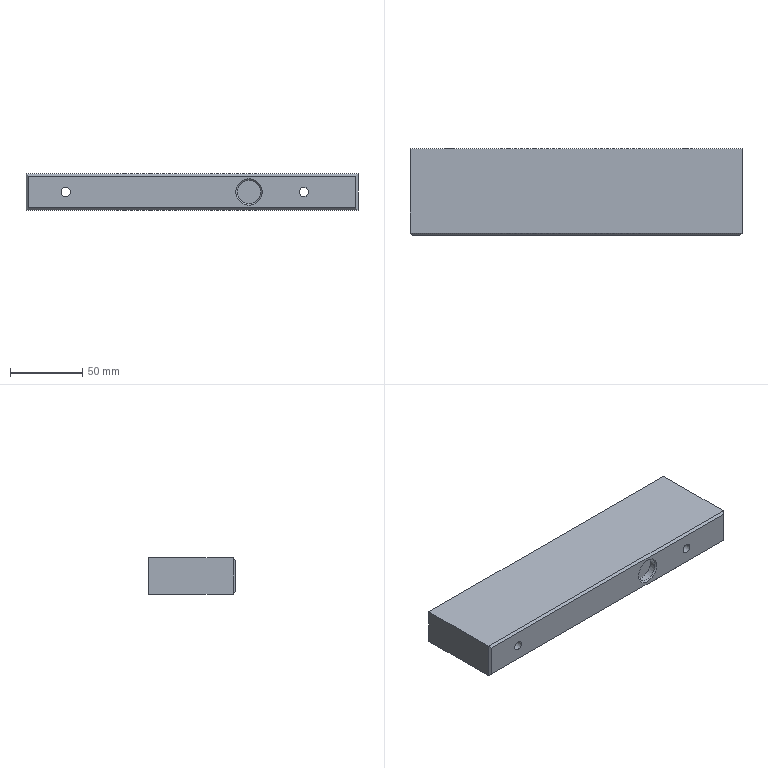NC program | NX | posted with a generic post | part box 230 x 60 x 25 mm
Whole program:
N10 G17 G21 G94 G90
(FLOOR_FACING_COPY_2_1 , TOOL : D63粗)
N12 T18 M6
N14 G53
N16 G17 G0 G90 X-156.5 Y0. B0. C0. S1600 M3
N18 G43 Z50. H18
N20 Z3.1
N22 G94 G1 Z0.1 F1000.
N24 X-146.5
N26 X146.5
N28 X156.5
N30 Z3.1
N32 G0 Z50.
N34 M5
(ADAPTIVE_MILLING , TOOL : D16CU)
N36 T01 M6
N38 G53
N40 G17 G0 G90 X-135.049 Y-29.091 B0. C0. S3000 M3
N42 G43 Z50. H1
N44 Z-23.
N46 G94 G1 X-134.899 Y-29.101 Z-23.937 F3000.
N48 X-134.75 Y-29.112 Z-24.308
N50 X-134.6 Y-29.122 Z-24.58
N52 X-134.45 Y-29.132 Z-24.8
N54 X-134.301 Y-29.142 Z-24.984
N56 X-134.151 Y-29.153 Z-25.142
N58 X-134.001 Y-29.163 Z-25.28
N60 X-133.852 Y-29.173 Z-25.4
N62 X-133.702 Y-29.184 Z-25.505
N64 X-133.552 Y-29.194 Z-25.598
N66 X-133.403 Y-29.204 Z-25.679
N68 X-133.253 Y-29.215 Z-25.75
N70 X-133.104 Y-29.225 Z-25.81
N72 X-132.954 Y-29.235 Z-25.862
N74 X-132.804 Y-29.245 Z-25.905
N76 X-132.655 Y-29.256 Z-25.939
N78 X-132.505 Y-29.266 Z-25.966
N80 X-132.355 Y-29.276 Z-25.985
N82 X-132.206 Y-29.287 Z-25.996
N84 X-132.056 Y-29.297 Z-26.
N86 X-129.709 Y-29.459
N88 G3 X-128.025 Y-28.217 R1.616
N90 X-127.719 Y-24.715 R19.992
N92 X-127.651 Y-13.97 R528.057
N94 G1 X-127.648 Y30.611
N96 G2 X-124.491 Y37.012 R8.791
N98 X-118.78 Y39.721 R12.771
N100 X-112.607 Y40.333 R33.389
N102 X-101.933 Y40.4 R573.424
N104 G1 X117.722
N106 G2 X124.165 Y37.332 R8.765
N108 X126.953 Y31.584 R12.699
N110 X127.58 Y25.456 R32.646
N112 X127.65 Y14.125 R538.765
N114 G1 X127.649 Y-30.591
N116 G2 X124.502 Y-36.997 R8.785
N118 X118.752 Y-39.725 R12.796
N120 X112.491 Y-40.336 R33.869
N122 X100.679 Y-40.4 R664.908
N124 G1 X-117.822 Y-40.399
N126 G2 X-124.235 Y-37.266 R8.778
N128 X-127.101 Y-30.561 R12.623
N130 X-127.336 Y-25.058 R41.411
N132 G1 X-127.301 Y-14.407
N134 X-127.3 Y28.293
N136 G2 X-122.512 Y37.044 R10.677
N138 X-116.175 Y39.467 R15.874
N140 X-109.289 Y39.995 R46.408
N142 X-97.477 Y40.05 R745.899
N144 G1 X115.428
N146 G2 X124.325 Y35.204 R10.699
N148 X126.702 Y28.994 R15.867
N150 X127.242 Y22.241 R45.
N152 X127.3 Y11.173 R708.797
N154 G1 X127.298 Y-28.328
N156 G2 X122.454 Y-37.08 R10.685
N158 X116.276 Y-39.448 R15.843
N160 X109.173 Y-39.997 R46.378
N162 X97.449 Y-40.05 R743.802
N164 G1 X-115.535 Y-40.049
N166 G2 X-124.65 Y-34.657 R10.654
N168 X-126.622 Y-28.481 R16.034
N170 X-126.945 Y-21.58 R58.208
N172 G1 X-126.951 Y-14.583
N174 X-126.95 Y26.28
N176 G2 X-120.661 Y37.088 R12.015
N178 X-114.157 Y39.176 R18.651
N180 X-106.828 Y39.651 R57.936
N182 X-94.928 Y39.699 R768.809
N184 G1 X113.284 Y39.7
N186 G2 X120.343 Y37.753 R12.31
N188 X125.289 Y31.377 R13.191
N190 X126.668 Y24.805 R23.956
N192 X126.939 Y15.887 R115.575
N194 G1 X126.949 Y8.668
N196 X126.948 Y-26.328
N198 G2 X120.708 Y-37.059 R12.003
N200 X114.078 Y-39.186 R18.692
N202 X106.661 Y-39.653 R59.426
N204 X95.548 Y-39.699 R739.332
N206 G1 X-113.392
N208 G2 X-120.464 Y-37.66 R12.075
N210 X-125.233 Y-31.186 R12.936
N212 X-126.423 Y-24.663 R24.39
N214 X-126.597 Y-16.004 R147.535
N216 G1 X-126.601 Y-11.191
N218 X-126.599 Y24.527
N220 G2 X-125.446 Y30.583 R14.572
N222 X-119.366 Y36.854 R13.13
N224 X-117.784 Y37.641 R5.968
N226 X-112.228 Y38.909 R22.581
N228 X-103.842 Y39.317 R80.649
N230 G1 X-92.905 Y39.349
N232 X111.752 Y39.347
N234 G2 X117.769 Y38.219 R14.63
N236 X124.325 Y31.659 R13.234
N238 X126.164 Y24.802 R21.871
N240 X126.574 Y16.153 R81.695
N242 G1 X126.599 Y6.528
N244 X126.598 Y-24.479
N246 G2 X125.533 Y-30.378 R14.74
N248 X119.085 Y-36.991 R13.16
N250 X112.244 Y-38.89 R21.425
N252 X104.253 Y-39.311 R73.777
N254 X93.141 Y-39.349 R763.66
N256 G1 X-111.772 Y-39.347
N258 G2 X-117.665 Y-38.254 R14.446
N260 X-124.175 Y-31.678 R12.94
N262 X-125.891 Y-24.966 R21.456
N264 X-126.227 Y-17.276 R79.847
N266 G1 X-126.25 Y-7.652
N268 X-126.249 Y22.822
N270 G2 X-125.556 Y28.312 R18.244
N272 X-122.168 Y33.868 R13.501
N274 X-120.762 Y35.764 R9.493
N276 X-118.699 Y37.262 R9.527
N278 X-115.22 Y38.181 R9.515
N280 X-103.672 Y38.952 R90.208
N282 X-91.16 Y38.998 R800.657
N284 G1 X110.927 Y38.993
N286 G2 X116.4 Y38.02 R16.228
N288 G1 X117.52 Y37.751
N290 G2 X119.791 Y36.593 R9.495
N292 X122.342 Y33.824 R11.401
N294 X125.436 Y26.122 R19.852
N296 X126.16 Y18.157 R50.149
N298 X126.249 Y4.245 R625.468
N300 G1 X126.247 Y-22.817
N302 G2 X125.58 Y-28.224 R18.356
N304 X118.784 Y-36.293 R13.58
N306 G3 X117.199 Y-37.262 R40.34
N308 G2 X114.774 Y-38.05 R9.495
N310 X105.722 Y-38.904 R55.451
N312 X91.11 Y-38.998 R646.625
N314 G1 X-110.134 Y-38.996
N316 G2 X-115.661 Y-38.259 R17.622
N318 X-123.418 Y-31.467 R13.355
N320 X-125.418 Y-24.563 R21.16
N322 X-125.864 Y-16.398 R70.739
N324 G1 X-125.9 Y-5.373
N326 X-125.899 Y25.727
N328 G2 X-125.359 Y27.572 R8.88
N330 X-122.936 Y32.078 R19.973
N332 G1 X-122.772 Y32.435
N334 G3 X-122.886 Y33.596 R1.603
N336 G1 X-123.29 Y34.391
N338 X-124.735 Y37.232 Z-25.9
N340 X-124.963 Y37.703 F15000.
N342 G2 X-124.629 Y39.363 R1.6
N344 G1 X-122.485 Y41.636
N346 G2 X-120.094 Y41.565 R1.6
N348 G1 X-119.75 Y41.154
N350 X-117.704 Y38.711 Z-26. F3000.
N352 G3 X-116.274 Y38.05 R1.644
N354 G2 X-113.555 Y38.173 R31.183
N356 X-97.124 Y38.64 R241.301
N358 G1 X-89.774 Y38.648
N360 X109.027 Y38.646
N362 G2 X114.03 Y38.15 R26.898
N364 X116.404 Y38.019 R13.509
N366 G3 X116.982 Y37.988 R1.678
N368 G1 X118.883 Y38.232
N370 G3 X119.296 Y41.328 R1.616
N372 G1 X119.157 Y41.385 Z-25.996
N374 X119.019 Y41.442 Z-25.985
N376 X118.88 Y41.5 Z-25.966
N378 X118.742 Y41.557 Z-25.939
N380 X118.603 Y41.615 Z-25.905
N382 X118.465 Y41.672 Z-25.862
N384 X118.326 Y41.73 Z-25.81
N386 X118.187 Y41.787 Z-25.75
N388 X118.049 Y41.844 Z-25.679
N390 X117.91 Y41.902 Z-25.598
N392 X117.772 Y41.959 Z-25.505
N394 X117.633 Y42.017 Z-25.4
N396 X117.495 Y42.074 Z-25.28
N398 X117.356 Y42.132 Z-25.142
N400 X117.217 Y42.189 Z-24.984
N402 X117.079 Y42.246 Z-24.8
N404 X116.94 Y42.304 Z-24.58
N406 X116.802 Y42.361 Z-24.308
N408 X116.663 Y42.419 Z-23.937
N410 X116.525 Y42.476 Z-23.
N412 G0 Z50.
N414 X-112.811 Y42.319
N416 Z-23.
N418 G1 X-112.96 Y42.307 Z-23.937
N420 X-113.11 Y42.296 Z-24.308
N422 X-113.259 Y42.284 Z-24.58
N424 X-113.409 Y42.272 Z-24.8
N426 X-113.558 Y42.26 Z-24.984
N428 X-113.708 Y42.248 Z-25.142
N430 X-113.857 Y42.237 Z-25.28
N432 X-114.007 Y42.225 Z-25.4
N434 X-114.156 Y42.213 Z-25.505
N436 X-114.306 Y42.201 Z-25.598
N438 X-114.455 Y42.19 Z-25.679
N440 X-114.605 Y42.178 Z-25.75
N442 X-114.755 Y42.166 Z-25.81
N444 X-114.904 Y42.154 Z-25.862
N446 X-115.054 Y42.143 Z-25.905
N448 X-115.203 Y42.131 Z-25.939
N450 X-115.353 Y42.119 Z-25.966
N452 X-115.502 Y42.107 Z-25.985
N454 X-115.652 Y42.096 Z-25.996
N456 X-115.801 Y42.084 Z-26.
N458 G3 X-116.413 Y39.035 R1.616
N460 G1 X-115.038 Y38.329
N462 G3 X-114.299 Y38.15 R1.631
N464 X-101.013 Y38.264 R625.418
N466 G1 X-88.676 Y38.298
N468 X108.718 Y38.288
N470 G2 X110.857 Y38.15 R143.224
N472 G1 X114.051
N474 G3 X114.539 Y41.274 R1.6
N476 G1 X111.469 Y42.131 Z-25.9
N478 X110.687 Y42.352 F15000.
N480 X109.902 Y42.561
N482 X109.613 Y42.588
N484 X-104.174
N486 X-104.391 Y42.571
N488 X-104.604 Y42.529
N490 X-106.003 Y42.139
N492 X-109.073 Y41.282 Z-26. F3000.
N494 G3 X-108.612 Y38.15 R1.6
N496 G1 X115.001
N498 G2 X117.52 Y37.751 R9.498
N500 X119.791 Y36.593 R9.495
N502 X121.594 Y34.789 R9.495
N504 X123.209 Y31.664 R18.055
N506 X125.502 Y22.308 R30.476
N508 X125.875 Y12.606 R111.361
N510 G1 X125.898 Y2.456
N512 X125.897 Y-23.091
N514 G2 X124.237 Y-29.753 R16.081
N516 X121.477 Y-33.427 R14.028
N518 X118.331 Y-36.559 R24.079
N520 G3 X119.756 Y-39.328 R1.6
N522 G1 X120.046 Y-39.226 Z-25.99
N524 X120.324 Y-39.095 Z-25.981
N526 X122.653 Y-38.002 Z-25.9
N528 X125.052 Y-36.876 F15000.
N530 G3 X125.503 Y-36.559 R1.673
N532 G1 X126.434 Y-35.616
N534 G3 X127.373 Y-34.267 R6.545
N536 X128.847 Y-31.237 R39.16
N538 X129.775 Y-28.682 R23.217
N540 X130.303 Y-25.909 R15.983
N542 X130.693 Y-18.974 R64.681
N544 G1 X130.67 Y11.341
N546 G3 X130.099 Y24.286 R154.907
N548 X129.641 Y28.411 R108.243
N550 G1 X129.19 Y31.843
N552 G3 X128.515 Y32.949 R1.602
N554 G1 X126.245 Y34.522
N556 X124.576 Y35.673 Z-25.964 F3000.
N558 G3 X123.463 Y35.887 Z-26. R1.6
N560 X122.262 Y33.699 R1.6
N562 G2 X123.068 Y31.472 R13.69
N564 X125.323 Y19.2 R44.866
N566 X125.541 Y7.741 R227.684
N568 G1 X125.548 Y0.916
N570 X125.546 Y-23.091
N572 G2 X122.844 Y-30.771 R16.786
N574 G1 X122.762 Y-30.973
N576 G3 X123.867 Y-32.881 R1.6
N578 X125.219 Y-32.668 Z-25.956 R1.612
N580 G1 X126.685 Y-31.669 Z-25.9
N582 X128.124 Y-30.689 F15000.
N584 G3 X128.824 Y-29.349 R1.601
N586 G1 X128.186 Y29.38
N588 G3 X127.93 Y30.23 R1.608
N590 G1 X127.024 Y31.634
N592 X125.603 Y33.825 Z-25.982 F3000.
N594 G3 X125.192 Y34.224 Z-26. R1.626
N596 X122.751 Y32.517 R1.6
N598 G2 X123.507 Y29.038 R104.994
N600 X125.069 Y16.153 R63.637
N602 X125.197 Y-0.471 R596.055
N604 G1 X125.196 Y-23.091
N606 G2 X123.345 Y-28.805 R21.054
N608 G3 X123.065 Y-29.593 R3.367
N610 X124.135 Y-31.286 R1.6
N612 X125.5 Y-31.132 Z-25.956 R1.612
N614 G1 X127.001 Y-30.198 Z-25.9
N616 X128.372 Y-29.346 F15000.
N618 G3 X129.127 Y-27.969 R1.601
N620 G1 X128.485 Y28.136
N622 G3 X128.206 Y29.02 R1.607
N624 G1 X127.105 Y30.634
N626 X126.511 Y31.51 Z-25.933 F3000.
N628 X125.907 Y32.378 Z-25.966
N630 G3 X125.027 Y32.953 Z-26. R1.6
N632 X123.05 Y31.274 R1.6
N634 X123.691 Y26.532 R43.68
N636 G2 X124.762 Y13.726 R86.847
N638 X124.847 Y-1.761 R828.191
N640 G1 Y-24.224
N642 G3 X125.024 Y-24.994 R1.777
N644 X127.731 Y-25.578 Z-25.9 R1.762
N646 X128.366 Y-24.168 R1.761 F15000.
N648 G1 X127.135 Y14.898
N650 X127.035 Y18.084 Z-26. F3000.
N652 X126.646 Y30.42
N654 G3 X123.132 Y30.227 R-1.76
N656 X123.527 Y25.528 R35.315
N658 G2 X124.443 Y11.085 R119.409
N660 X124.497 Y-2.915 R858.892
N662 G1 X124.495 Y-24.24
N664 G2 X124.025 Y-25.878 R8.007
N666 G3 X123.164 Y-28.364 R29.548
N668 G1 X123.049 Y-29.776
N670 G2 X122.261 Y-32.201 R9.495
N672 X121.451 Y-33.458 R9.564
N674 G3 X123.35 Y-35.944 R1.6
N676 X123.808 Y-35.629 Z-25.983 R2.04
N678 G1 X125.832 Y-33.95 Z-25.9
N680 X126.934 Y-33.035 F15000.
N682 G3 X127.512 Y-31.833 R1.601
N684 G1 X128.585 Y26.162
N686 G3 X128.284 Y27.125 R1.605
N688 G1 X127.146 Y28.709
N690 X126.572 Y29.51 Z-25.931 F3000.
N692 X125.99 Y30.306 Z-25.962
N694 G3 X124.956 Y30.886 Z-26. R1.6
N696 X123.15 Y29.299 R1.6
N698 X123.377 Y24.19 R39.929
N700 G2 X124.119 Y7.678 R172.876
N702 G1 X124.146 Y-4.047
N704 X124.145 Y-24.235
N706 G2 X123.742 Y-25.61 R5.562
N708 G3 X123.154 Y-27.534 R11.235
N710 G1 X123.15 Y-28.501
N712 G3 X124.938 Y-30.089 R1.6
N714 X126.053 Y-29.429 Z-25.958 R1.617
N716 G1 X127.128 Y-27.919 Z-25.9
N718 X128.288 Y-26.291 F15000.
N720 G3 X128.585 Y-25.363 R1.605
N722 G1 Y24.324
N724 G3 X128.288 Y25.252 R1.605
N726 G1 X127.143 Y26.86
N728 X126.573 Y27.665 Z-25.931 F3000.
N730 X125.995 Y28.463 Z-25.962
N732 G3 X124.963 Y29.048 Z-26. R1.6
N734 X123.15 Y27.462 R1.6
N736 X123.385 Y19.991 R82.008
N738 G2 X123.785 Y3.592 R279.443
N740 G1 X123.795 Y-3.671
N742 X123.794 Y-23.596
N744 G2 X123.372 Y-25.302 R13.468
N746 G3 X123.15 Y-26.319 R9.169
N748 G1 Y-27.631
N750 G3 X124.924 Y-29.222 R1.6
N752 X126.048 Y-28.567 Z-25.958 R1.617
N754 G1 X127.128 Y-27.068 Z-25.9
N756 X128.283 Y-25.465 F15000.
N758 G3 X128.585 Y-24.493 R1.604
N760 G1 X127.588 Y20.137
N762 X127.569 Y20.334
N764 X127.53 Y20.528
N766 X127.138 Y21.944
N768 X126.288 Y25.016 Z-26. F3000.
N770 G3 X123.15 Y24.574 R1.6
N772 X123.314 Y13.375 R250.496
N774 G2 X123.445 Y-5.875 R878.023
N776 G1 X123.444 Y-22.343
N778 X123.15 Y-24.267
N780 Y-26.323
N782 G3 X124.922 Y-27.914 R1.6
N784 X126.047 Y-27.26 Z-25.958 R1.617
N786 G1 X127.128 Y-25.762 Z-25.9
N788 X128.283 Y-24.164 F15000.
N790 G3 X128.585 Y-23.185 R1.604
N792 G1 X127.588 Y15.149
N794 X127.569 Y15.343
N796 X127.53 Y15.534
N798 X127.138 Y16.953
N800 X126.289 Y20.025 Z-26. F3000.
N802 G3 X123.15 Y19.587 R1.6
N804 G1 Y-28.501
N806 G2 X122.751 Y-31.02 R9.498
N808 X121.593 Y-33.291 R9.495
N810 X118.289 Y-36.594 R24.549
N812 X116.017 Y-37.751 R9.495
N814 X113.499 Y-38.15 R9.5
N816 X105.177 Y-38.549 R371.9
N818 X90.39 Y-38.648 R687.061
N820 G1 X-109.512 Y-38.643
N822 G2 X-113.978 Y-38.112 R20.32
N824 G1 X-114.776 Y-38.049
N826 G2 X-117.201 Y-37.261 R9.495
N828 X-120.154 Y-34.923 R11.339
N830 X-121.772 Y-33.04 R21.59
N832 X-124.785 Y-25.253 R20.298
N834 X-125.458 Y-17.634 R50.883
N836 X-125.549 Y-3.372 R630.493
N838 G1 X-125.55 Y25.716
N840 G3 X-125.744 Y26.48 R1.614
N842 X-128.422 Y26.686 Z-25.9 R1.602
N844 G1 X-128.551 Y26.485 F15000.
N846 X-128.651 Y26.27
N848 X-130.522 Y21.198
N850 G3 X-130.621 Y20.644 R1.667
N852 G1 Y-21.799
N854 G3 X-128.042 Y-31.881 R20.999
N856 G1 X-125.464 Y-36.593
N858 G3 X-124.679 Y-37.3 R1.604
N860 G1 X-122.424 Y-38.246
N862 X-119.871 Y-39.313 Z-25.987 F3000.
N864 X-119.669 Y-39.371 Z-25.993
N866 X-119.461 Y-39.404 Z-26.
N868 G3 X-118.291 Y-36.593 R1.6
N870 G2 X-121.594 Y-33.289 R24.549
N872 X-122.751 Y-31.017 R9.495
N874 X-124.972 Y-19.622 R39.167
N876 X-125.192 Y-8.775 R203.517
N878 G1 X-125.199 Y-1.688
N880 X-125.198 Y25.737
N882 G2 X-124.59 Y27.743 R8.889
N884 X-123.133 Y30.914 R65.379
N886 G1 X-123.056 Y31.21
N888 G3 X-124.119 Y32.906 R1.6
N890 X-125.489 Y32.755 Z-25.955 R1.612
N892 G1 X-126.986 Y31.825 Z-25.9
N894 X-128.362 Y30.971 F15000.
N896 G3 X-129.118 Y29.586 R1.601
N898 G1 X-128.186 Y-27.88
N900 G3 X-127.931 Y-28.72 R1.609
N902 G1 X-127.024 Y-30.129
N904 X-125.604 Y-32.324 Z-25.982 F3000.
N906 G3 X-125.195 Y-32.721 Z-26. R1.626
N908 X-122.751 Y-31.017 R1.6
N910 G2 X-124.348 Y-22.202 R76.08
N912 X-124.813 Y-12.066 R107.136
N914 G1 X-124.849 Y-0.254
N916 Y25.683
N918 G3 X-125.026 Y26.453 R1.777
N920 X-127.734 Y27.037 Z-25.9 R1.762
N922 X-128.368 Y25.626 R1.761 F15000.
N924 G1 X-127.135 Y-12.361
N926 X-127.032 Y-15.547 Z-26. F3000.
N928 X-126.563 Y-29.969
N930 G3 X-123.05 Y-29.774 R-1.76
N932 X-123.617 Y-25.054 R57.533
N934 G2 X-124.432 Y-13.19 R95.402
N936 X-124.498 Y1.072 R830.537
N938 G1 X-124.499 Y25.697
N940 G2 X-124.061 Y27.342 R7.375
N942 G3 X-123.162 Y29.94 R65.002
N944 G1 X-123.049 Y31.276
N946 G2 X-122.261 Y33.701 R9.495
N948 G1 X-122.101 Y33.962
N950 G3 X-122.629 Y36.162 R1.6
N952 X-124.827 Y35.639 R1.6
N954 G1 X-125.228 Y34.988
N956 X-126.903 Y32.275 Z-25.9
N958 X-127.148 Y31.884 F15000.
N960 X-127.38 Y31.485
N962 G3 X-127.536 Y30.824 R1.624
N964 G1 X-128.574 Y-25.502
N966 G3 X-128.289 Y-26.443 R1.605
N968 G1 X-127.145 Y-28.094
N970 X-125.994 Y-29.747 Z-25.963 F3000.
N972 G3 X-125.013 Y-30.341 Z-26. R1.6
N974 X-123.139 Y-28.64 R1.6
N976 X-123.431 Y-24.024 R40.198
N978 G2 X-124.117 Y-9.522 R146.966
N980 G1 X-124.148 Y2.028
N982 Y25.691
N984 G2 X-123.834 Y26.872 R4.272
N986 G3 X-123.155 Y29.083 R14.218
N988 G1 X-123.147 Y30.044
N990 G3 X-124.989 Y31.751 R1.6
N992 X-126.061 Y31.075 Z-25.959 R1.617
N994 G1 X-127.128 Y29.521 Z-25.9
N996 X-128.301 Y27.812 F15000.
N998 G3 X-128.581 Y26.906 R1.606
N1000 G1 X-128.585 Y-24.443
N1002 G3 X-128.288 Y-25.371 R1.605
N1004 G1 X-127.143 Y-26.978
N1006 X-126.573 Y-27.783 Z-25.931 F3000.
N1008 X-125.995 Y-28.582 Z-25.962
N1010 G3 X-124.964 Y-29.166 Z-26. R1.6
N1012 X-123.15 Y-27.581 R1.6
N1014 X-123.387 Y-20.666 R73.311
N1016 G2 X-123.787 Y-5.055 R252.437
N1018 G1 X-123.797 Y3.432
N1020 X-123.798 Y25.082
N1022 G2 X-123.549 Y26.19 R6.066
N1024 G3 X-123.15 Y27.881 R12.189
N1026 G1 Y29.193
N1028 G3 X-124.925 Y30.783 R1.6
N1030 X-126.048 Y30.128 Z-25.958 R1.617
N1032 G1 X-127.128 Y28.629 Z-25.9
N1034 X-128.284 Y27.024 F15000.
N1036 G3 X-128.585 Y26.055 R1.604
N1038 G1 X-127.588 Y-20.649
N1040 X-127.569 Y-20.847
N1042 X-127.53 Y-21.042
N1044 X-127.138 Y-22.457
N1046 X-126.288 Y-25.529 Z-26. F3000.
N1048 G3 X-123.15 Y-25.087 R1.6
N1050 X-123.317 Y-14.341 R233.59
N1052 G2 X-123.447 Y4.383 R827.581
N1054 G1 Y23.821
N1056 X-123.15 Y25.803
N1058 Y27.903
N1060 G3 X-124.923 Y29.494 R1.6
N1062 X-126.048 Y28.839 Z-25.958 R1.617
N1064 G1 X-127.128 Y27.341 Z-25.9
N1066 X-128.283 Y25.741 F15000.
N1068 G3 X-128.585 Y24.765 R1.604
N1070 G1 X-127.588 Y-15.968
N1072 X-127.569 Y-16.163
N1074 X-127.53 Y-16.355
N1076 X-127.138 Y-17.773
N1078 X-126.288 Y-20.845 Z-26. F3000.
N1080 G3 X-123.15 Y-20.406 R1.6
N1082 G1 Y25.838
N1084 G3 X-123.31 Y26.539 R1.635
N1086 G1 X-124.063 Y28.102
N1088 G3 X-127.134 Y27.4 R1.616
N1090 G1 Y27.25 Z-25.996
N1092 Y27.1 Z-25.985
N1094 Y26.95 Z-25.966
N1096 Y26.8 Z-25.939
N1098 Y26.65 Z-25.905
N1100 Y26.5 Z-25.862
N1102 Y26.35 Z-25.81
N1104 Y26.2 Z-25.75
N1106 Y26.05 Z-25.679
N1108 Y25.9 Z-25.598
N1110 Y25.75 Z-25.505
N1112 Y25.6 Z-25.4
N1114 Y25.45 Z-25.28
N1116 Y25.3 Z-25.142
N1118 Y25.15 Z-24.984
N1120 Y25. Z-24.8
N1122 Y24.85 Z-24.58
N1124 Y24.7 Z-24.308
N1126 Y24.55 Z-23.937
N1128 Y24.4 Z-23.
N1130 G0 Z50.
N1132 X120.452 Y-40.228
N1134 Z-23.
N1136 G1 X120.314 Y-40.285 Z-23.937
N1138 X120.175 Y-40.342 Z-24.308
N1140 X120.037 Y-40.4 Z-24.58
N1142 X119.898 Y-40.457 Z-24.8
N1144 X119.759 Y-40.515 Z-24.984
N1146 X119.621 Y-40.572 Z-25.142
N1148 X119.482 Y-40.629 Z-25.28
N1150 X119.344 Y-40.687 Z-25.4
N1152 X119.205 Y-40.744 Z-25.505
N1154 X119.066 Y-40.802 Z-25.598
N1156 X118.928 Y-40.859 Z-25.679
N1158 X118.789 Y-40.916 Z-25.75
N1160 X118.651 Y-40.974 Z-25.81
N1162 X118.512 Y-41.031 Z-25.862
N1164 X118.373 Y-41.088 Z-25.905
N1166 X118.235 Y-41.146 Z-25.939
N1168 X118.096 Y-41.203 Z-25.966
N1170 X117.958 Y-41.261 Z-25.985
N1172 X117.819 Y-41.318 Z-25.996
N1174 X117.681 Y-41.375 Z-26.
N1176 G2 X115.576 Y-40.516 R1.616
N1178 G1 X114.986 Y-39.132
N1180 G3 X113.499 Y-38.15 R1.616
N1182 X100.689 Y-38.264 R613.19
N1184 G1 X88.439 Y-38.298
N1186 X-107.536 Y-38.296
N1188 G2 X-110.718 Y-38.15 R38.751
N1190 G1 X-113.501
N1192 X-113.98 Y-38.112
N1194 G3 X-114.526 Y-41.251 R1.6
N1196 G1 X-114.371 Y-41.293
N1198 X-111.295 Y-42.131 Z-25.9
N1200 X-110.562 Y-42.334 F15000.
N1202 X-109.825 Y-42.525
N1204 X-109.543 Y-42.55
N1206 X103.812 Y-42.588
N1208 X104.029 Y-42.571
N1210 X104.242 Y-42.529
N1212 X105.639 Y-42.139
N1214 X108.71 Y-41.282 Z-26. F3000.
N1216 G3 X108.249 Y-38.15 R1.6
N1218 G1 X-110.719
N1220 G3 X-112.329 Y-39.622 R1.616
N1222 G1 X-112.553 Y-42.134
N1224 X-112.567 Y-42.284 Z-25.996
N1226 X-112.58 Y-42.433 Z-25.985
N1228 X-112.593 Y-42.583 Z-25.966
N1230 X-112.607 Y-42.732 Z-25.939
N1232 X-112.62 Y-42.882 Z-25.905
N1234 X-112.633 Y-43.031 Z-25.862
N1236 X-112.647 Y-43.18 Z-25.81
N1238 X-112.66 Y-43.33 Z-25.75
N1240 X-112.673 Y-43.479 Z-25.679
N1242 X-112.687 Y-43.629 Z-25.598
N1244 X-112.7 Y-43.778 Z-25.505
N1246 X-112.713 Y-43.927 Z-25.4
N1248 X-112.727 Y-44.077 Z-25.28
N1250 X-112.74 Y-44.226 Z-25.142
N1252 X-112.753 Y-44.376 Z-24.984
N1254 X-112.767 Y-44.525 Z-24.8
N1256 X-112.78 Y-44.674 Z-24.58
N1258 X-112.793 Y-44.824 Z-24.308
N1260 X-112.807 Y-44.973 Z-23.937
N1262 X-112.82 Y-45.123 Z-23.
N1264 G0 Z50.
N1266 M5
(PLANAR_MILL_COPY , TOOL : D8点钻)
N1268 T03 M6
N1270 G53
N1272 G17 G0 G90 X-119.165 Y-30.452 B0. C0. S4500 M3
N1274 G43 Z50. H3
N1276 Z-2.5
N1278 G94 G3 X-117.6 Y-28.5 R2. F800.
N1280 G1 Y30.
N1282 G2 X-115. Y32.6 R2.6
N1284 G1 X115.
N1286 G2 X117.6 Y30. R2.6
N1288 G1 Y-28.5
N1290 G2 X115. Y-31.1 R2.6
N1292 G1 X-115.
N1294 G2 X-117.6 Y-28.5 R2.6
N1296 G3 X-119.6 Y-26.5 R2.
N1298 G0 Z50.
N1300 M5
(PLANAR_MILL_COPY_COPY_1 , TOOL : 4倒角)
N1302 T19 M6
N1304 G53
N1306 G17 G0 G90 X116.93 Y-31.774 B0. C0. S4500 M3
N1308 G43 Z50. H19
N1310 Z-1.8
N1312 G94 G3 X115. Y-30.3 R2. F800.
N1314 G1 X-115.
N1316 G2 X-116.8 Y-28.5 R1.8
N1318 G1 Y30.
N1320 G2 X-115. Y31.8 R1.8
N1322 G1 X115.
N1324 G2 X116.8 Y30. R1.8
N1326 G1 Y-28.5
N1328 G2 X115. Y-30.3 R1.8
N1330 G3 X113. Y-32.3 R2.
N1332 G0 Z50.
N1334 M5
(PLANAR_MILL , TOOL : D16.)
N1336 T02 M6
N1338 G53
N1340 G17 G0 G90 X-124.831 Y-30.49 B0. C0. S1300 M3
N1342 G43 Z50. H2
N1344 Z-25.5
N1346 G94 G3 X-123.03 Y-28.5 R2. F400.
N1348 G1 Y30.
N1350 G2 X-115. Y38.03 R8.03
N1352 G1 X115.
N1354 G2 X123.03 Y30. R8.03
N1356 G1 Y-28.5
N1358 G2 X120.678 Y-34.178 R8.03
N1360 G1 X119.178 Y-35.678
N1362 G2 X113.5 Y-38.03 R8.03
N1364 G1 X-113.5
N1366 G2 X-119.178 Y-35.678 R8.03
N1368 G1 X-120.678 Y-34.178
N1370 G2 X-123.03 Y-28.5 R8.03
N1372 G3 X-125.03 Y-26.5 R2.
N1374 G1 X-124.83 Y-30.493
N1376 G3 X-123. Y-28.5 R2.
N1378 G1 Y30.
N1380 G2 X-115. Y38. R8.
N1382 G1 X115.
N1384 G2 X123. Y30. R8.
N1386 G1 Y-28.5
N1388 G2 X120.657 Y-34.157 R8.
N1390 G1 X119.157 Y-35.657
N1392 G2 X113.5 Y-38. R8.
N1394 G1 X-113.5
N1396 G2 X-119.157 Y-35.657 R8.
N1398 G1 X-120.657 Y-34.157
N1400 G2 X-123. Y-28.5 R8.
N1402 G3 X-125.03 Y-26.5 R2.
N1404 G0 Z50.
N1406 M5
(FLOOR_FACING_COPY_2_1_COPY , TOOL : D63精)
N1408 T20 M6
N1410 G53
N1412 G17 G0 G90 X-156.5 Y0. B0. C0. S1600 M3
N1414 G43 Z50. H20
N1416 Z3.
N1418 G94 G1 Z0. F400.
N1420 X-146.5
N1422 X146.5
N1424 X156.5
N1426 Z3.
N1428 G0 Z50.
N1430 M5
(FLOOR_FACING_COPY_2_1_COPY_1 , TOOL : D63粗)
N1432 T18 M6
N1434 G53
N1436 G17 G0 G90 X-156.5 Y0. B0. C0. S1600 M3
N1438 G43 Z50. H18
N1440 Z8.2
N1442 G94 G1 Z5.2 F1000.
N1444 X-146.5
N1446 X146.5
N1448 X156.5
N1450 Z8.2
N1452 G0 Z8.5
N1454 X-156.5
N1456 Z7.9
N1458 G1 Z4.9
N1460 X-146.5
N1462 X146.5
N1464 X156.5
N1466 Z7.9
N1468 G0 Z8.2
N1470 X-156.5
N1472 Z7.6
N1474 G1 Z4.6
N1476 X-146.5
N1478 X146.5
N1480 X156.5
N1482 Z7.6
N1484 G0 Z7.9
N1486 X-156.5
N1488 Z7.3
N1490 G1 Z4.3
N1492 X-146.5
N1494 X146.5
N1496 X156.5
N1498 Z7.3
N1500 G0 Z7.6
N1502 X-156.5
N1504 Z7.
N1506 G1 Z4.
N1508 X-146.5
N1510 X146.5
N1512 X156.5
N1514 Z7.
N1516 G0 Z7.3
N1518 X-156.5
N1520 Z6.7
N1522 G1 Z3.7
N1524 X-146.5
N1526 X146.5
N1528 X156.5
N1530 Z6.7
N1532 G0 Z7.
N1534 X-156.5
N1536 Z6.4
N1538 G1 Z3.4
N1540 X-146.5
N1542 X146.5
N1544 X156.5
N1546 Z6.4
N1548 G0 Z6.7
N1550 X-156.5
N1552 Z6.1
N1554 G1 Z3.1
N1556 X-146.5
N1558 X146.5
N1560 X156.5
N1562 Z6.1
N1564 G0 Z6.4
N1566 X-156.5
N1568 Z5.8
N1570 G1 Z2.8
N1572 X-146.5
N1574 X146.5
N1576 X156.5
N1578 Z5.8
N1580 G0 Z6.1
N1582 X-156.5
N1584 Z5.5
N1586 G1 Z2.5
N1588 X-146.5
N1590 X146.5
N1592 X156.5
N1594 Z5.5
N1596 G0 Z8.5
N1598 X-156.5
N1600 Z5.2
N1602 G1 Z2.2
N1604 X-146.5
N1606 X146.5
N1608 X156.5
N1610 Z5.2
N1612 G0 Z8.5
N1614 X-156.5
N1616 Z4.9
N1618 G1 Z1.9
N1620 X-146.5
N1622 X146.5
N1624 X156.5
N1626 Z4.9
N1628 G0 Z8.5
N1630 X-156.5
N1632 Z4.6
N1634 G1 Z1.6
N1636 X-146.5
N1638 X146.5
N1640 X156.5
N1642 Z4.6
N1644 G0 Z8.5
N1646 X-156.5
N1648 Z4.3
N1650 G1 Z1.3
N1652 X-146.5
N1654 X146.5
N1656 X156.5
N1658 Z4.3
N1660 G0 Z8.5
N1662 X-156.5
N1664 Z4.
N1666 G1 Z1.
N1668 X-146.5
N1670 X146.5
N1672 X156.5
N1674 Z4.
N1676 G0 Z8.5
N1678 X-156.5
N1680 Z3.7
N1682 G1 Z0.7
N1684 X-146.5
N1686 X146.5
N1688 X156.5
N1690 Z3.7
N1692 G0 Z8.5
N1694 X-156.5
N1696 Z3.4
N1698 G1 Z0.4
N1700 X-146.5
N1702 X146.5
N1704 X156.5
N1706 Z3.4
N1708 G0 Z8.5
N1710 X-156.5
N1712 Z3.1
N1714 G1 Z0.1
N1716 X-146.5
N1718 X146.5
N1720 X156.5
N1722 Z3.1
N1724 G0 Z50.
N1726 M5
(FLOOR_FACING_COPY_2_1_COPY_COPY , TOOL : D63精)
N1728 T20 M6
N1730 G53
N1732 G17 G0 G90 X-156.5 Y0. B0. C0. S1600 M3
N1734 G43 Z50. H20
N1736 Z3.
N1738 G94 G1 Z0. F500.
N1740 X-146.5
N1742 X146.5
N1744 X156.5
N1746 Z3.
N1748 G0 Z50.
(FLOOR_FACING_COPY_2_1_COPY_COPY_COPY , TOOL : D63精)
N1750 X-156.5
N1752 Z3.
N1754 G1 Z0.
N1756 X-146.5
N1758 X146.5
N1760 X156.5
N1762 Z3.
N1764 G0 Z50.
N1766 M5
(PLANAR_MILL_COPY_COPY , TOOL : D8点钻)
N1768 T03 M6
N1770 G53
N1772 G17 G0 G90 X-119.056 Y-30.45 B0. C0. S4500 M3
N1774 G43 Z50. H3
N1776 Z-2.5
N1778 G94 G3 X-117.5 Y-28.5 R2. F1200.
N1780 G1 Y30.
N1782 G2 X-115. Y32.5 R2.5
N1784 G1 X115.
N1786 G2 X117.5 Y30. R2.5
N1788 G1 Y-28.5
N1790 G2 X115. Y-31. R2.5
N1792 G1 X-115.
N1794 G2 X-117.5 Y-28.5 R2.5
N1796 G3 X-119.5 Y-26.5 R2.
N1798 G0 Z50.
N1800 M5
(PLANAR_MILL_COPY_COPY_1_COPY , TOOL : 4倒角)
N1802 T19 M6
N1804 G53
N1806 G17 G0 G90 X116.93 Y-31.774 B0. C0. S4500 M3
N1808 G43 Z50. H19
N1810 Z-1.8
N1812 G94 G3 X115. Y-30.3 R2. F800.
N1814 G1 X-115.
N1816 G2 X-116.8 Y-28.5 R1.8
N1818 G1 Y30.
N1820 G2 X-115. Y31.8 R1.8
N1822 G1 X115.
N1824 G2 X116.8 Y30. R1.8
N1826 G1 Y-28.5
N1828 G2 X115. Y-30.3 R1.8
N1830 G3 X113. Y-32.3 R2.
N1832 G0 Z50.
N1834 M5
(SPOT_FACING , TOOL : D8点钻)
N1836 T03 M6
N1838 G53
N1840 G17 G0 G90 X-87.5 Y0. B0. C0. S1500 M3
N1842 G43 Z30. H3
N1844 G94 G82 G98 Z-3.4 B-180. C-180. F100. P200 R2.
N1846 X39.5
N1848 X77.5
N1850 G80
N1852 G0 X77.5 Y0. Z30.
N1854 M5
(PECK_DRILLING_COPY_1 , TOOL : Z5.)
N1856 T09 M6
N1858 G53
N1860 G17 G0 G90 X-87.5 Y0. B0. C0. S2500 M3
N1862 G43 Z30. H9
N1864 G94 G83 G99 Z-30. B-180. C-180. F130. Q2. R3.
N1866 X77.5
N1868 G80
N1870 G0 X77.5 Y0. Z30.
N1872 M5
(PECK_DRILLING , TOOL : Z6.5)
N1874 T21 M6
N1876 G53
N1878 G17 G0 G90 X-87.5 Y0. B0. C0. S1200 M3
N1880 G43 Z30. H21
N1882 G94 G83 G99 Z-65. B-180. C-180. F80. Q2. R3.
N1884 X77.5
N1886 G80
N1888 G0 X77.5 Y0. Z30.
(PECK_DRILLING_COPY , TOOL : Z6.5)
N1890 X39.5
N1892 G83 Z-5.5 F80. Q2. R3.
N1894 G80
N1896 G0 X39.5 Y0. Z30.
N1898 M5
(HOLE_MILLING , TOOL : D10.)
N1900 T24 M6
N1902 G53
N1904 G17 G0 G90 X39.5 Y0. B0. C0. S2800 M3
N1906 G43 Z30. H24
N1908 Z0.5 B-180. C-180.
N1910 G94 G3 X41.035 Y-1.535 R1.535 F800.
N1912 X42.57 Y0. R1.535
N1914 X42.57 Y0. Z0.3 I-3.07 J0.
N1916 X42.57 Y0. Z0.1 I-3.07 J0.
N1918 X42.57 Y0. Z-0.1 I-3.07 J0.
N1920 X42.57 Y0. Z-0.3 I-3.07 J0.
N1922 X42.57 Y0. Z-0.5 I-3.07 J0.
N1924 X42.57 Y0. Z-0.7 I-3.07 J0.
N1926 X42.57 Y0. Z-0.9 I-3.07 J0.
N1928 X42.57 Y0. Z-1.1 I-3.07 J0.
N1930 X42.57 Y0. Z-1.3 I-3.07 J0.
N1932 X42.57 Y0. Z-1.5 I-3.07 J0.
N1934 X42.57 Y0. Z-1.7 I-3.07 J0.
N1936 X42.57 Y0. Z-1.9 I-3.07 J0.
N1938 X42.57 Y0. Z-2.1 I-3.07 J0.
N1940 X42.57 Y0. Z-2.3 I-3.07 J0.
N1942 X42.57 Y0. Z-2.5 I-3.07 J0.
N1944 X42.57 Y0. Z-2.7 I-3.07 J0.
N1946 X42.57 Y0. Z-2.9 I-3.07 J0.
N1948 X42.57 Y0. Z-3.1 I-3.07 J0.
N1950 X42.57 Y0. Z-3.3 I-3.07 J0.
N1952 X42.57 Y0. Z-3.5 I-3.07 J0.
N1954 X42.57 Y0. Z-3.7 I-3.07 J0.
N1956 X42.57 Y0. Z-3.9 I-3.07 J0.
N1958 X42.57 Y0. Z-4.1 I-3.07 J0.
N1960 X42.57 Y0. Z-4.3 I-3.07 J0.
N1962 X42.57 Y0. Z-4.5 I-3.07 J0.
N1964 X42.57 Y0. Z-4.7 I-3.07 J0.
N1966 X42.57 Y0. Z-4.9 I-3.07 J0.
N1968 X42.57 Y0. Z-5.1 I-3.07 J0.
N1970 X42.57 Y0. Z-5.3 I-3.07 J0.
N1972 X41.984 Y-1.805 Z-5.48 R-3.07
N1974 X41.305 Y2.484 R3.07
N1976 X41.984 Y-1.805 R-3.07
N1978 X41.644 Y0.34 R1.535
N1980 X39.5 Y0. R1.535
N1982 G0 Z30.
(HOLE_MILLING_COPY , TOOL : D10.)
N1984 S2500
N1986 Z-5.5
N1988 G3 X41.05 Y-1.55 R1.55 F150.
N1990 X42.6 Y0. R1.55
N1992 X39.5 Y3.1 R3.1
N1994 X42.6 Y0. R-3.1
N1996 X41.05 Y1.55 R1.55
N1998 X39.5 Y0. R1.55
N2000 G0 Z30.
N2002 M5
(PLANAR_MILL_1 , TOOL : D8点钻)
N2004 T03 M6
N2006 G53
N2008 G17 G0 G90 X39.5 Y4.9 B0. C0. S4500 M3
N2010 G43 Z30. H3
N2012 Z1. B-180. C-180.
N2014 G94 G1 Z-2. F300.
N2016 Y6.9
N2018 G3 X32.6 Y0. R6.9
N2020 X39.5 Y6.9 R-6.9
N2022 G1 Y4.9
N2024 Z1.
N2026 G0 Z30.
N2028 M5
(PLANAR_MILL_1_COPY , TOOL : 4倒角)
N2030 T19 M6
N2032 G53
N2034 G17 G0 G90 X39.5 Y5.3 B0. C0. S4500 M3
N2036 G43 Z30. H19
N2038 Z1.3 B-180. C-180.
N2040 G94 G1 Z-1.7 F300.
N2042 G41 Y7.3
N2044 G3 X32.2 Y0. R7.3
N2046 X39.5 Y7.3 R-7.3
N2048 G40
N2050 G1 Y5.3
N2052 Z1.3
N2054 G0 Z30.
N2056 M5
N2058 M2